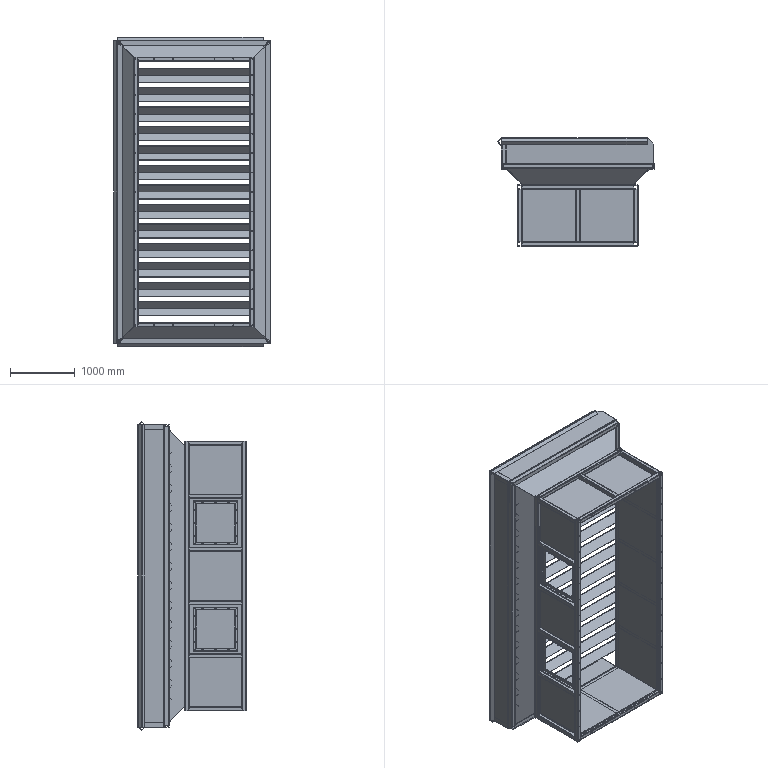Part | SolidWorks | features ReferencePattern 53, LocalLPattern 8, MirrorCompFeat 3 | 100 solids | 1903 faces | box 2415 x 1670 x 4774 mm | volume 225195392 mm3 | plane 948 | cylinder 571 | cone 336 | torus 48 | commonest cylinder face diameters 13 x248 12 x136 24 x88 18 x48 6 x18 4 x16